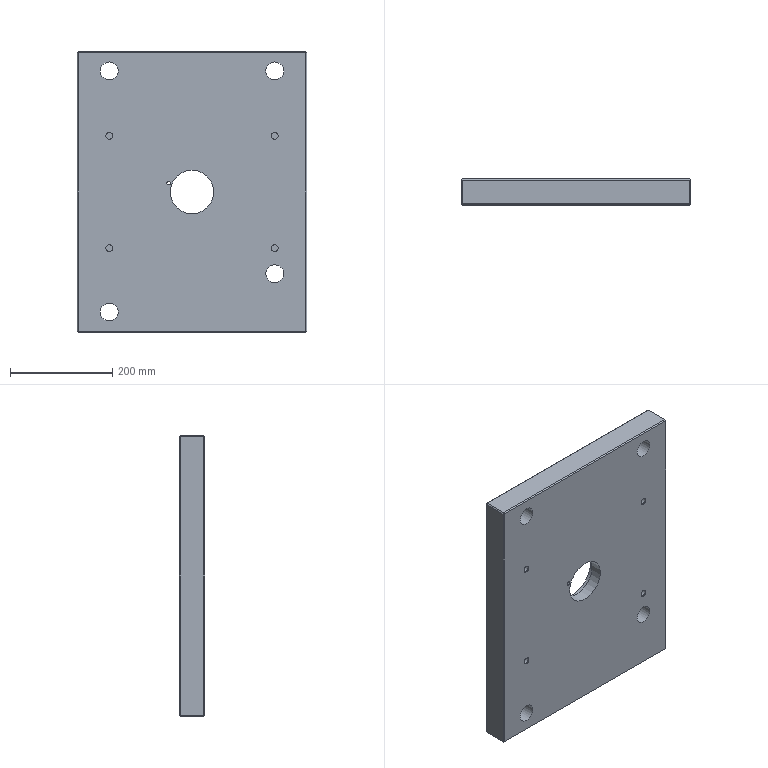Part | STEP file | TOP-CLAMP-PLATE_id506_x_t | 1 solid | 58 faces | box 450 x 50 x 550 mm | volume 11584870 mm3 | plane 29 | cylinder 21 | cone 8 | commonest cylinder face diameters 13.2 x4 16 x4 35 x4 40 x4 7 x1 12 x1
STEP:
#1=CARTESIAN_POINT('',(0.,160.5,84.487));
#2=VERTEX_POINT('',#1);
#3=CARTESIAN_POINT('',(0.,160.5,0.));
#4=DIRECTION('',(0.,1.,0.));
#5=DIRECTION('',(0.,0.,1.));
#6=AXIS2_PLACEMENT_3D('',#3,#4,#5);
#7=CIRCLE('',#6,84.487);
#8=EDGE_CURVE('',#2,#2,#7,.T.);
#9=ORIENTED_EDGE('',*,*,#8,.F.);
#10=EDGE_LOOP('',(#9));
#11=FACE_BOUND('',#10,.T.);
#12=CARTESIAN_POINT('',(0.,175.5,84.487));
#13=VERTEX_POINT('',#12);
#14=CARTESIAN_POINT('',(0.,175.5,0.));
#15=DIRECTION('',(0.,-1.,0.));
#16=DIRECTION('',(0.,0.,1.));
#17=AXIS2_PLACEMENT_3D('',#14,#15,#16);
#18=CIRCLE('',#17,84.487);
#19=EDGE_CURVE('',#13,#13,#18,.T.);
#20=ORIENTED_EDGE('',*,*,#19,.F.);
#21=EDGE_LOOP('',(#20));
#22=FACE_BOUND('',#21,.T.);
#23=CARTESIAN_POINT('',(0.,123.,0.));
#24=DIRECTION('',(0.,1.,0.));
#25=DIRECTION('',(0.,0.,1.));
#26=AXIS2_PLACEMENT_3D('',#23,#24,#25);
#27=CYLINDRICAL_SURFACE('',#26,84.487);
#28=ADVANCED_FACE('',(#11,#22),#27,.F.);
#29=CARTESIAN_POINT('',(-162.,147.5,103.));
#30=VERTEX_POINT('',#29);
#31=CARTESIAN_POINT('',(-162.,147.5,110.));
#32=DIRECTION('',(0.,-1.,0.));
#33=DIRECTION('',(0.,0.,-1.));
#34=AXIS2_PLACEMENT_3D('',#31,#32,#33);
#35=CIRCLE('',#34,7.);
#36=EDGE_CURVE('',#30,#30,#35,.T.);
#37=ORIENTED_EDGE('',*,*,#36,.T.);
#38=EDGE_LOOP('',(#37));
#39=FACE_OUTER_BOUND('',#38,.T.);
#40=CARTESIAN_POINT('',(-162.,147.5,110.));
#41=DIRECTION('',(0.,-1.,0.));
#42=DIRECTION('',(0.,0.,-1.));
#43=AXIS2_PLACEMENT_3D('',#40,#41,#42);
#44=PLANE('',#43);
#45=ADVANCED_FACE('',(#39),#44,.T.);
#46=CARTESIAN_POINT('',(-162.,147.5,-117.));
#47=VERTEX_POINT('',#46);
#48=CARTESIAN_POINT('',(-162.,147.5,-110.));
#49=DIRECTION('',(0.,-1.,0.));
#50=DIRECTION('',(0.,0.,-1.));
#51=AXIS2_PLACEMENT_3D('',#48,#49,#50);
#52=CIRCLE('',#51,7.);
#53=EDGE_CURVE('',#47,#47,#52,.T.);
#54=ORIENTED_EDGE('',*,*,#53,.T.);
#55=EDGE_LOOP('',(#54));
#56=FACE_OUTER_BOUND('',#55,.T.);
#57=CARTESIAN_POINT('',(-162.,147.5,-110.));
#58=DIRECTION('',(0.,1.,0.));
#59=DIRECTION('',(0.,0.,1.));
#60=AXIS2_PLACEMENT_3D('',#57,#58,#59);
#61=PLANE('',#60);
#62=ADVANCED_FACE('',(#56),#61,.F.);
#63=CARTESIAN_POINT('',(162.,147.5,103.));
#64=VERTEX_POINT('',#63);
#65=CARTESIAN_POINT('',(162.,147.5,110.));
#66=DIRECTION('',(0.,-1.,0.));
#67=DIRECTION('',(0.,0.,-1.));
#68=AXIS2_PLACEMENT_3D('',#65,#66,#67);
#69=CIRCLE('',#68,7.);
#70=EDGE_CURVE('',#64,#64,#69,.T.);
#71=ORIENTED_EDGE('',*,*,#70,.T.);
#72=EDGE_LOOP('',(#71));
#73=FACE_OUTER_BOUND('',#72,.T.);
#74=CARTESIAN_POINT('',(162.,147.5,110.));
#75=DIRECTION('',(0.,1.,0.));
#76=DIRECTION('',(0.,0.,1.));
#77=AXIS2_PLACEMENT_3D('',#74,#75,#76);
#78=PLANE('',#77);
#79=ADVANCED_FACE('',(#73),#78,.F.);
#80=CARTESIAN_POINT('',(162.,147.5,-117.));
#81=VERTEX_POINT('',#80);
#82=CARTESIAN_POINT('',(162.,147.5,-110.));
#83=DIRECTION('',(0.,-1.,0.));
#84=DIRECTION('',(0.,0.,-1.));
#85=AXIS2_PLACEMENT_3D('',#82,#83,#84);
#86=CIRCLE('',#85,7.);
#87=EDGE_CURVE('',#81,#81,#86,.T.);
#88=ORIENTED_EDGE('',*,*,#87,.T.);
#89=EDGE_LOOP('',(#88));
#90=FACE_OUTER_BOUND('',#89,.T.);
#91=CARTESIAN_POINT('',(162.,147.5,-110.));
#92=DIRECTION('',(0.,-1.,0.));
#93=DIRECTION('',(0.,0.,-1.));
#94=AXIS2_PLACEMENT_3D('',#91,#92,#93);
#95=PLANE('',#94);
#96=ADVANCED_FACE('',(#90),#95,.T.);
#97=ORIENTED_EDGE('',*,*,#19,.T.);
#98=EDGE_LOOP('',(#97));
#99=FACE_BOUND('',#98,.T.);
#100=CARTESIAN_POINT('',(162.,175.5,257.));
#101=VERTEX_POINT('',#100);
#102=CARTESIAN_POINT('',(162.,175.5,237.));
#103=DIRECTION('',(0.,-1.,0.));
#104=DIRECTION('',(0.,0.,1.));
#105=AXIS2_PLACEMENT_3D('',#102,#103,#104);
#106=CIRCLE('',#105,20.);
#107=EDGE_CURVE('',#101,#101,#106,.T.);
#108=ORIENTED_EDGE('',*,*,#107,.T.);
#109=EDGE_LOOP('',(#108));
#110=FACE_BOUND('',#109,.T.);
#111=CARTESIAN_POINT('',(-162.,175.5,257.));
#112=VERTEX_POINT('',#111);
#113=CARTESIAN_POINT('',(-162.,175.5,237.));
#114=DIRECTION('',(0.,-1.,0.));
#115=DIRECTION('',(0.,0.,1.));
#116=AXIS2_PLACEMENT_3D('',#113,#114,#115);
#117=CIRCLE('',#116,20.);
#118=EDGE_CURVE('',#112,#112,#117,.T.);
#119=ORIENTED_EDGE('',*,*,#118,.T.);
#120=EDGE_LOOP('',(#119));
#121=FACE_BOUND('',#120,.T.);
#122=CARTESIAN_POINT('',(-162.,175.5,-215.));
#123=VERTEX_POINT('',#122);
#124=CARTESIAN_POINT('',(-162.,175.5,-235.));
#125=DIRECTION('',(0.,-1.,0.));
#126=DIRECTION('',(0.,0.,1.));
#127=AXIS2_PLACEMENT_3D('',#124,#125,#126);
#128=CIRCLE('',#127,20.);
#129=EDGE_CURVE('',#123,#123,#128,.T.);
#130=ORIENTED_EDGE('',*,*,#129,.T.);
#131=EDGE_LOOP('',(#130));
#132=FACE_BOUND('',#131,.T.);
#133=CARTESIAN_POINT('',(162.,175.5,-140.));
#134=VERTEX_POINT('',#133);
#135=CARTESIAN_POINT('',(162.,175.5,-160.));
#136=DIRECTION('',(0.,-1.,0.));
#137=DIRECTION('',(0.,0.,1.));
#138=AXIS2_PLACEMENT_3D('',#135,#136,#137);
#139=CIRCLE('',#138,20.);
#140=EDGE_CURVE('',#134,#134,#139,.T.);
#141=ORIENTED_EDGE('',*,*,#140,.T.);
#142=EDGE_LOOP('',(#141));
#143=FACE_BOUND('',#142,.T.);
#144=CARTESIAN_POINT('',(-223.,175.5,273.));
#145=VERTEX_POINT('',#144);
#146=CARTESIAN_POINT('',(-223.,175.5,-273.));
#147=VERTEX_POINT('',#146);
#148=CARTESIAN_POINT('',(-223.,175.5,273.));
#149=DIRECTION('',(0.,0.,-1.));
#150=VECTOR('',#149,1.);
#151=LINE('',#148,#150);
#152=EDGE_CURVE('',#145,#147,#151,.T.);
#153=ORIENTED_EDGE('',*,*,#152,.F.);
#154=CARTESIAN_POINT('',(223.,175.5,273.));
#155=VERTEX_POINT('',#154);
#156=CARTESIAN_POINT('',(-225.,175.5,273.));
#157=DIRECTION('',(-1.,0.,0.));
#158=VECTOR('',#157,1.);
#159=LINE('',#156,#158);
#160=EDGE_CURVE('',#155,#145,#159,.T.);
#161=ORIENTED_EDGE('',*,*,#160,.F.);
#162=CARTESIAN_POINT('',(223.,175.5,-273.));
#163=VERTEX_POINT('',#162);
#164=CARTESIAN_POINT('',(223.,175.5,273.));
#165=DIRECTION('',(0.,0.,1.));
#166=VECTOR('',#165,1.);
#167=LINE('',#164,#166);
#168=EDGE_CURVE('',#163,#155,#167,.T.);
#169=ORIENTED_EDGE('',*,*,#168,.F.);
#170=CARTESIAN_POINT('',(-225.,175.5,-273.));
#171=DIRECTION('',(-1.,0.,0.));
#172=VECTOR('',#171,1.);
#173=LINE('',#170,#172);
#174=EDGE_CURVE('',#163,#147,#173,.T.);
#175=ORIENTED_EDGE('',*,*,#174,.T.);
#176=EDGE_LOOP('',(#153,#161,#169,#175));
#177=FACE_BOUND('',#176,.T.);
#178=CARTESIAN_POINT('',(-225.,175.5,275.));
#179=DIRECTION('',(0.,1.,0.));
#180=DIRECTION('',(0.,0.,1.));
#181=AXIS2_PLACEMENT_3D('',#178,#179,#180);
#182=PLANE('',#181);
#183=ADVANCED_FACE('',(#99,#110,#121,#132,#143,#177),#182,.T.);
#184=CARTESIAN_POINT('',(-48.524,160.5,12.058));
#185=VERTEX_POINT('',#184);
#186=CARTESIAN_POINT('',(-44.286,160.5,23.21));
#187=VERTEX_POINT('',#186);
#188=CARTESIAN_POINT('',(0.,160.5,0.));
#189=DIRECTION('',(0.,-1.,0.));
#190=DIRECTION('',(0.,0.,1.));
#191=AXIS2_PLACEMENT_3D('',#188,#189,#190);
#192=CIRCLE('',#191,50.);
#193=EDGE_CURVE('',#185,#187,#192,.T.);
#194=ORIENTED_EDGE('',*,*,#193,.T.);
#195=CARTESIAN_POINT('',(-45.804,160.5,17.406));
#196=DIRECTION('',(0.,-1.,0.));
#197=DIRECTION('',(0.,0.,1.));
#198=AXIS2_PLACEMENT_3D('',#195,#196,#197);
#199=CIRCLE('',#198,6.);
#200=EDGE_CURVE('',#187,#185,#199,.T.);
#201=ORIENTED_EDGE('',*,*,#200,.T.);
#202=EDGE_LOOP('',(#194,#201));
#203=FACE_BOUND('',#202,.T.);
#204=ORIENTED_EDGE('',*,*,#8,.T.);
#205=EDGE_LOOP('',(#204));
#206=FACE_BOUND('',#205,.T.);
#207=CARTESIAN_POINT('',(0.,160.5,0.));
#208=DIRECTION('',(0.,1.,0.));
#209=DIRECTION('',(0.,0.,1.));
#210=AXIS2_PLACEMENT_3D('',#207,#208,#209);
#211=PLANE('',#210);
#212=ADVANCED_FACE('',(#203,#206),#211,.T.);
#213=ORIENTED_EDGE('',*,*,#36,.F.);
#214=EDGE_LOOP('',(#213));
#215=FACE_BOUND('',#214,.T.);
#216=CARTESIAN_POINT('',(-162.,147.,102.));
#217=VERTEX_POINT('',#216);
#218=CARTESIAN_POINT('',(-162.,147.,110.));
#219=DIRECTION('',(0.,-1.,0.));
#220=DIRECTION('',(0.,0.,-1.));
#221=AXIS2_PLACEMENT_3D('',#218,#219,#220);
#222=CIRCLE('',#221,8.);
#223=EDGE_CURVE('',#217,#217,#222,.T.);
#224=ORIENTED_EDGE('',*,*,#223,.T.);
#225=EDGE_LOOP('',(#224));
#226=FACE_BOUND('',#225,.T.);
#227=CARTESIAN_POINT('',(-162.,147.,110.));
#228=DIRECTION('',(0.,-1.,0.));
#229=DIRECTION('',(0.,0.,-1.));
#230=AXIS2_PLACEMENT_3D('',#227,#228,#229);
#231=CONICAL_SURFACE('',#230,8.,63.435);
#232=ADVANCED_FACE('',(#215,#226),#231,.F.);
#233=ORIENTED_EDGE('',*,*,#53,.F.);
#234=EDGE_LOOP('',(#233));
#235=FACE_BOUND('',#234,.T.);
#236=CARTESIAN_POINT('',(-162.,147.,-102.));
#237=VERTEX_POINT('',#236);
#238=CARTESIAN_POINT('',(-162.,147.,-110.));
#239=DIRECTION('',(0.,-1.,0.));
#240=DIRECTION('',(0.,0.,1.));
#241=AXIS2_PLACEMENT_3D('',#238,#239,#240);
#242=CIRCLE('',#241,8.);
#243=EDGE_CURVE('',#237,#237,#242,.T.);
#244=ORIENTED_EDGE('',*,*,#243,.T.);
#245=EDGE_LOOP('',(#244));
#246=FACE_BOUND('',#245,.T.);
#247=CARTESIAN_POINT('',(-162.,147.,-110.));
#248=DIRECTION('',(0.,-1.,0.));
#249=DIRECTION('',(0.,0.,-1.));
#250=AXIS2_PLACEMENT_3D('',#247,#248,#249);
#251=CONICAL_SURFACE('',#250,8.,63.435);
#252=ADVANCED_FACE('',(#235,#246),#251,.F.);
#253=ORIENTED_EDGE('',*,*,#70,.F.);
#254=EDGE_LOOP('',(#253));
#255=FACE_BOUND('',#254,.T.);
#256=CARTESIAN_POINT('',(162.,147.,118.));
#257=VERTEX_POINT('',#256);
#258=CARTESIAN_POINT('',(162.,147.,110.));
#259=DIRECTION('',(0.,-1.,0.));
#260=DIRECTION('',(0.,0.,1.));
#261=AXIS2_PLACEMENT_3D('',#258,#259,#260);
#262=CIRCLE('',#261,8.);
#263=EDGE_CURVE('',#257,#257,#262,.T.);
#264=ORIENTED_EDGE('',*,*,#263,.T.);
#265=EDGE_LOOP('',(#264));
#266=FACE_BOUND('',#265,.T.);
#267=CARTESIAN_POINT('',(162.,147.,110.));
#268=DIRECTION('',(0.,-1.,0.));
#269=DIRECTION('',(0.,0.,-1.));
#270=AXIS2_PLACEMENT_3D('',#267,#268,#269);
#271=CONICAL_SURFACE('',#270,8.,63.435);
#272=ADVANCED_FACE('',(#255,#266),#271,.F.);
#273=CARTESIAN_POINT('',(162.,147.,-118.));
#274=VERTEX_POINT('',#273);
#275=CARTESIAN_POINT('',(162.,147.,-110.));
#276=DIRECTION('',(0.,-1.,0.));
#277=DIRECTION('',(0.,0.,-1.));
#278=AXIS2_PLACEMENT_3D('',#275,#276,#277);
#279=CIRCLE('',#278,8.);
#280=EDGE_CURVE('',#274,#274,#279,.T.);
#281=ORIENTED_EDGE('',*,*,#280,.T.);
#282=EDGE_LOOP('',(#281));
#283=FACE_BOUND('',#282,.T.);
#284=ORIENTED_EDGE('',*,*,#87,.F.);
#285=EDGE_LOOP('',(#284));
#286=FACE_BOUND('',#285,.T.);
#287=CARTESIAN_POINT('',(162.,147.,-110.));
#288=DIRECTION('',(0.,-1.,0.));
#289=DIRECTION('',(0.,0.,-1.));
#290=AXIS2_PLACEMENT_3D('',#287,#288,#289);
#291=CONICAL_SURFACE('',#290,8.,63.435);
#292=ADVANCED_FACE('',(#283,#286),#291,.F.);
#293=CARTESIAN_POINT('',(-224.,174.5,274.));
#294=VERTEX_POINT('',#293);
#295=CARTESIAN_POINT('',(-223.,175.5,273.));
#296=DIRECTION('',(-0.5774,-0.5774,0.5774));
#297=VECTOR('',#296,1.);
#298=LINE('',#295,#297);
#299=EDGE_CURVE('',#145,#294,#298,.T.);
#300=ORIENTED_EDGE('',*,*,#299,.F.);
#301=ORIENTED_EDGE('',*,*,#152,.T.);
#302=CARTESIAN_POINT('',(-224.,174.5,-274.));
#303=VERTEX_POINT('',#302);
#304=CARTESIAN_POINT('',(-223.,175.5,-273.));
#305=DIRECTION('',(-0.5774,-0.5774,-0.5774));
#306=VECTOR('',#305,1.);
#307=LINE('',#304,#306);
#308=EDGE_CURVE('',#147,#303,#307,.T.);
#309=ORIENTED_EDGE('',*,*,#308,.T.);
#310=CARTESIAN_POINT('',(-225.,173.5,-273.));
#311=VERTEX_POINT('',#310);
#312=CARTESIAN_POINT('',(-224.,174.5,-274.));
#313=DIRECTION('',(-0.5774,-0.5774,0.5774));
#314=VECTOR('',#313,1.);
#315=LINE('',#312,#314);
#316=EDGE_CURVE('',#303,#311,#315,.T.);
#317=ORIENTED_EDGE('',*,*,#316,.T.);
#318=CARTESIAN_POINT('',(-225.,173.5,273.));
#319=VERTEX_POINT('',#318);
#320=CARTESIAN_POINT('',(-225.,173.5,275.));
#321=DIRECTION('',(0.,0.,-1.));
#322=VECTOR('',#321,1.);
#323=LINE('',#320,#322);
#324=EDGE_CURVE('',#319,#311,#323,.T.);
#325=ORIENTED_EDGE('',*,*,#324,.F.);
#326=CARTESIAN_POINT('',(-224.,174.5,274.));
#327=DIRECTION('',(-0.5774,-0.5774,-0.5774));
#328=VECTOR('',#327,1.);
#329=LINE('',#326,#328);
#330=EDGE_CURVE('',#294,#319,#329,.T.);
#331=ORIENTED_EDGE('',*,*,#330,.F.);
#332=EDGE_LOOP('',(#300,#301,#309,#317,#325,#331));
#333=FACE_OUTER_BOUND('',#332,.T.);
#334=CARTESIAN_POINT('',(-223.,175.5,273.));
#335=DIRECTION('',(-0.7071,0.7071,0.));
#336=DIRECTION('',(-0.7071,-0.7071,0.));
#337=AXIS2_PLACEMENT_3D('',#334,#335,#336);
#338=PLANE('',#337);
#339=ADVANCED_FACE('',(#333),#338,.T.);
#340=CARTESIAN_POINT('',(-225.,127.5,-273.));
#341=VERTEX_POINT('',#340);
#342=CARTESIAN_POINT('',(-224.,126.5,-274.));
#343=VERTEX_POINT('',#342);
#344=CARTESIAN_POINT('',(-225.,127.5,-273.));
#345=DIRECTION('',(0.5774,-0.5774,-0.5774));
#346=VECTOR('',#345,1.);
#347=LINE('',#344,#346);
#348=EDGE_CURVE('',#341,#343,#347,.T.);
#349=ORIENTED_EDGE('',*,*,#348,.F.);
#350=CARTESIAN_POINT('',(-225.,125.5,-273.));
#351=DIRECTION('',(0.,-1.,0.));
#352=VECTOR('',#351,1.);
#353=LINE('',#350,#352);
#354=EDGE_CURVE('',#311,#341,#353,.T.);
#355=ORIENTED_EDGE('',*,*,#354,.F.);
#356=ORIENTED_EDGE('',*,*,#316,.F.);
#357=CARTESIAN_POINT('',(-223.,173.5,-275.));
#358=VERTEX_POINT('',#357);
#359=CARTESIAN_POINT('',(-224.,174.5,-274.));
#360=DIRECTION('',(0.5774,-0.5774,-0.5774));
#361=VECTOR('',#360,1.);
#362=LINE('',#359,#361);
#363=EDGE_CURVE('',#303,#358,#362,.T.);
#364=ORIENTED_EDGE('',*,*,#363,.T.);
#365=CARTESIAN_POINT('',(-223.,127.5,-275.));
#366=VERTEX_POINT('',#365);
#367=CARTESIAN_POINT('',(-223.,60.,-275.));
#368=DIRECTION('',(0.,1.,0.));
#369=VECTOR('',#368,1.);
#370=LINE('',#367,#369);
#371=EDGE_CURVE('',#366,#358,#370,.T.);
#372=ORIENTED_EDGE('',*,*,#371,.F.);
#373=CARTESIAN_POINT('',(-224.,126.5,-274.));
#374=DIRECTION('',(0.5774,0.5774,-0.5774));
#375=VECTOR('',#374,1.);
#376=LINE('',#373,#375);
#377=EDGE_CURVE('',#343,#366,#376,.T.);
#378=ORIENTED_EDGE('',*,*,#377,.F.);
#379=EDGE_LOOP('',(#349,#355,#356,#364,#372,#378));
#380=FACE_OUTER_BOUND('',#379,.T.);
#381=CARTESIAN_POINT('',(-223.,127.5,-275.));
#382=DIRECTION('',(0.7071,0.,0.7071));
#383=DIRECTION('',(0.7071,0.,-0.7071));
#384=AXIS2_PLACEMENT_3D('',#381,#382,#383);
#385=PLANE('',#384);
#386=ADVANCED_FACE('',(#380),#385,.F.);
#387=ORIENTED_EDGE('',*,*,#308,.F.);
#388=ORIENTED_EDGE('',*,*,#174,.F.);
#389=CARTESIAN_POINT('',(224.,174.5,-274.));
#390=VERTEX_POINT('',#389);
#391=CARTESIAN_POINT('',(224.,174.5,-274.));
#392=DIRECTION('',(-0.5774,0.5774,0.5774));
#393=VECTOR('',#392,1.);
#394=LINE('',#391,#393);
#395=EDGE_CURVE('',#390,#163,#394,.T.);
#396=ORIENTED_EDGE('',*,*,#395,.F.);
#397=CARTESIAN_POINT('',(223.,173.5,-275.));
#398=VERTEX_POINT('',#397);
#399=CARTESIAN_POINT('',(224.,174.5,-274.));
#400=DIRECTION('',(-0.5774,-0.5774,-0.5774));
#401=VECTOR('',#400,1.);
#402=LINE('',#399,#401);
#403=EDGE_CURVE('',#390,#398,#402,.T.);
#404=ORIENTED_EDGE('',*,*,#403,.T.);
#405=CARTESIAN_POINT('',(200.,173.5,-275.));
#406=DIRECTION('',(1.,0.,0.));
#407=VECTOR('',#406,1.);
#408=LINE('',#405,#407);
#409=EDGE_CURVE('',#358,#398,#408,.T.);
#410=ORIENTED_EDGE('',*,*,#409,.F.);
#411=ORIENTED_EDGE('',*,*,#363,.F.);
#412=EDGE_LOOP('',(#387,#388,#396,#404,#410,#411));
#413=FACE_OUTER_BOUND('',#412,.T.);
#414=CARTESIAN_POINT('',(-225.,173.5,-275.));
#415=DIRECTION('',(0.,-0.7071,0.7071));
#416=DIRECTION('',(0.,-0.7071,-0.7071));
#417=AXIS2_PLACEMENT_3D('',#414,#415,#416);
#418=PLANE('',#417);
#419=ADVANCED_FACE('',(#413),#418,.F.);
#420=CARTESIAN_POINT('',(225.,173.5,-273.));
#421=VERTEX_POINT('',#420);
#422=CARTESIAN_POINT('',(225.,173.5,-273.));
#423=DIRECTION('',(-0.5774,0.5774,-0.5774));
#424=VECTOR('',#423,1.);
#425=LINE('',#422,#424);
#426=EDGE_CURVE('',#421,#390,#425,.T.);
#427=ORIENTED_EDGE('',*,*,#426,.F.);
#428=CARTESIAN_POINT('',(225.,127.5,-273.));
#429=VERTEX_POINT('',#428);
#430=CARTESIAN_POINT('',(225.,175.5,-273.));
#431=DIRECTION('',(0.,1.,0.));
#432=VECTOR('',#431,1.);
#433=LINE('',#430,#432);
#434=EDGE_CURVE('',#429,#421,#433,.T.);
#435=ORIENTED_EDGE('',*,*,#434,.F.);
#436=CARTESIAN_POINT('',(224.,126.5,-274.));
#437=VERTEX_POINT('',#436);
#438=CARTESIAN_POINT('',(224.,126.5,-274.));
#439=DIRECTION('',(0.5774,0.5774,0.5774));
#440=VECTOR('',#439,1.);
#441=LINE('',#438,#440);
#442=EDGE_CURVE('',#437,#429,#441,.T.);
#443=ORIENTED_EDGE('',*,*,#442,.F.);
#444=CARTESIAN_POINT('',(223.,127.5,-275.));
#445=VERTEX_POINT('',#444);
#446=CARTESIAN_POINT('',(223.,127.5,-275.));
#447=DIRECTION('',(0.5774,-0.5774,0.5774));
#448=VECTOR('',#447,1.);
#449=LINE('',#446,#448);
#450=EDGE_CURVE('',#445,#437,#449,.T.);
#451=ORIENTED_EDGE('',*,*,#450,.F.);
#452=CARTESIAN_POINT('',(223.,60.,-275.));
#453=DIRECTION('',(0.,-1.,0.));
#454=VECTOR('',#453,1.);
#455=LINE('',#452,#454);
#456=EDGE_CURVE('',#398,#445,#455,.T.);
#457=ORIENTED_EDGE('',*,*,#456,.F.);
#458=ORIENTED_EDGE('',*,*,#403,.F.);
#459=EDGE_LOOP('',(#427,#435,#443,#451,#457,#458));
#460=FACE_OUTER_BOUND('',#459,.T.);
#461=CARTESIAN_POINT('',(223.,175.5,-275.));
#462=DIRECTION('',(-0.7071,0.,0.7071));
#463=DIRECTION('',(0.7071,0.,0.7071));
#464=AXIS2_PLACEMENT_3D('',#461,#462,#463);
#465=PLANE('',#464);
#466=ADVANCED_FACE('',(#460),#465,.F.);
#467=CARTESIAN_POINT('',(225.,173.5,273.));
#468=VERTEX_POINT('',#467);
#469=CARTESIAN_POINT('',(224.,174.5,274.));
#470=VERTEX_POINT('',#469);
#471=CARTESIAN_POINT('',(225.,173.5,273.));
#472=DIRECTION('',(-0.5774,0.5774,0.5774));
#473=VECTOR('',#472,1.);
#474=LINE('',#471,#473);
#475=EDGE_CURVE('',#468,#470,#474,.T.);
#476=ORIENTED_EDGE('',*,*,#475,.F.);
#477=CARTESIAN_POINT('',(225.,173.5,275.));
#478=DIRECTION('',(0.,0.,1.));
#479=VECTOR('',#478,1.);
#480=LINE('',#477,#479);
#481=EDGE_CURVE('',#421,#468,#480,.T.);
#482=ORIENTED_EDGE('',*,*,#481,.F.);
#483=ORIENTED_EDGE('',*,*,#426,.T.);
#484=ORIENTED_EDGE('',*,*,#395,.T.);
#485=ORIENTED_EDGE('',*,*,#168,.T.);
#486=CARTESIAN_POINT('',(224.,174.5,274.));
#487=DIRECTION('',(-0.5774,0.5774,-0.5774));
#488=VECTOR('',#487,1.);
#489=LINE('',#486,#488);
#490=EDGE_CURVE('',#470,#155,#489,.T.);
#491=ORIENTED_EDGE('',*,*,#490,.F.);
#492=EDGE_LOOP('',(#476,#482,#483,#484,#485,#491));
#493=FACE_OUTER_BOUND('',#492,.T.);
#494=CARTESIAN_POINT('',(225.,173.5,273.));
#495=DIRECTION('',(0.7071,0.7071,0.));
#496=DIRECTION('',(-0.7071,0.7071,0.));
#497=AXIS2_PLACEMENT_3D('',#494,#495,#496);
#498=PLANE('',#497);
#499=ADVANCED_FACE('',(#493),#498,.T.);
#500=CARTESIAN_POINT('',(-224.,126.5,274.));
#501=VERTEX_POINT('',#500);
#502=CARTESIAN_POINT('',(-223.,127.5,275.));
#503=VERTEX_POINT('',#502);
#504=CARTESIAN_POINT('',(-224.,126.5,274.));
#505=DIRECTION('',(0.5774,0.5774,0.5774));
#506=VECTOR('',#505,1.);
#507=LINE('',#504,#506);
#508=EDGE_CURVE('',#501,#503,#507,.T.);
#509=ORIENTED_EDGE('',*,*,#508,.T.);
#510=CARTESIAN_POINT('',(-223.,173.5,275.));
#511=VERTEX_POINT('',#510);
#512=CARTESIAN_POINT('',(-223.,90.5,275.));
#513=DIRECTION('',(0.,1.,0.));
#514=VECTOR('',#513,1.);
#515=LINE('',#512,#514);
#516=EDGE_CURVE('',#503,#511,#515,.T.);
#517=ORIENTED_EDGE('',*,*,#516,.T.);
#518=CARTESIAN_POINT('',(-224.,174.5,274.));
#519=DIRECTION('',(0.5774,-0.5774,0.5774));
#520=VECTOR('',#519,1.);
#521=LINE('',#518,#520);
#522=EDGE_CURVE('',#294,#511,#521,.T.);
#523=ORIENTED_EDGE('',*,*,#522,.F.);
#524=ORIENTED_EDGE('',*,*,#330,.T.);
#525=CARTESIAN_POINT('',(-225.,127.5,273.));
#526=VERTEX_POINT('',#525);
#527=CARTESIAN_POINT('',(-225.,125.5,273.));
#528=DIRECTION('',(0.,1.,0.));
#529=VECTOR('',#528,1.);
#530=LINE('',#527,#529);
#531=EDGE_CURVE('',#526,#319,#530,.T.);
#532=ORIENTED_EDGE('',*,*,#531,.F.);
#533=CARTESIAN_POINT('',(-225.,127.5,273.));
#534=DIRECTION('',(0.5774,-0.5774,0.5774));
#535=VECTOR('',#534,1.);
#536=LINE('',#533,#535);
#537=EDGE_CURVE('',#526,#501,#536,.T.);
#538=ORIENTED_EDGE('',*,*,#537,.T.);
#539=EDGE_LOOP('',(#509,#517,#523,#524,#532,#538));
#540=FACE_OUTER_BOUND('',#539,.T.);
#541=CARTESIAN_POINT('',(-223.,127.5,275.));
#542=DIRECTION('',(-0.7071,0.,0.7071));
#543=DIRECTION('',(0.7071,0.,0.7071));
#544=AXIS2_PLACEMENT_3D('',#541,#542,#543);
#545=PLANE('',#544);
#546=ADVANCED_FACE('',(#540),#545,.T.);
#547=ORIENTED_EDGE('',*,*,#522,.T.);
#548=CARTESIAN_POINT('',(223.,173.5,275.));
#549=VERTEX_POINT('',#548);
#550=CARTESIAN_POINT('',(-200.,173.5,275.));
#551=DIRECTION('',(1.,0.,0.));
#552=VECTOR('',#551,1.);
#553=LINE('',#550,#552);
#554=EDGE_CURVE('',#511,#549,#553,.T.);
#555=ORIENTED_EDGE('',*,*,#554,.T.);
#556=CARTESIAN_POINT('',(224.,174.5,274.));
#557=DIRECTION('',(-0.5774,-0.5774,0.5774));
#558=VECTOR('',#557,1.);
#559=LINE('',#556,#558);
#560=EDGE_CURVE('',#470,#549,#559,.T.);
#561=ORIENTED_EDGE('',*,*,#560,.F.);
#562=ORIENTED_EDGE('',*,*,#490,.T.);
#563=ORIENTED_EDGE('',*,*,#160,.T.);
#564=ORIENTED_EDGE('',*,*,#299,.T.);
#565=EDGE_LOOP('',(#547,#555,#561,#562,#563,#564));
#566=FACE_OUTER_BOUND('',#565,.T.);
#567=CARTESIAN_POINT('',(-225.,173.5,275.));
#568=DIRECTION('',(0.,0.7071,0.7071));
#569=DIRECTION('',(0.,-0.7071,0.7071));
#570=AXIS2_PLACEMENT_3D('',#567,#568,#569);
#571=PLANE('',#570);
#572=ADVANCED_FACE('',(#566),#571,.T.);
#573=ORIENTED_EDGE('',*,*,#560,.T.);
#574=CARTESIAN_POINT('',(223.,127.5,275.));
#575=VERTEX_POINT('',#574);
#576=CARTESIAN_POINT('',(223.,90.5,275.));
#577=DIRECTION('',(0.,-1.,0.));
#578=VECTOR('',#577,1.);
#579=LINE('',#576,#578);
#580=EDGE_CURVE('',#549,#575,#579,.T.);
#581=ORIENTED_EDGE('',*,*,#580,.T.);
#582=CARTESIAN_POINT('',(224.,126.5,274.));
#583=VERTEX_POINT('',#582);
#584=CARTESIAN_POINT('',(223.,127.5,275.));
#585=DIRECTION('',(0.5774,-0.5774,-0.5774));
#586=VECTOR('',#585,1.);
#587=LINE('',#584,#586);
#588=EDGE_CURVE('',#575,#583,#587,.T.);
#589=ORIENTED_EDGE('',*,*,#588,.T.);
#590=CARTESIAN_POINT('',(225.,127.5,273.));
#591=VERTEX_POINT('',#590);
#592=CARTESIAN_POINT('',(224.,126.5,274.));
#593=DIRECTION('',(0.5774,0.5774,-0.5774));
#594=VECTOR('',#593,1.);
#595=LINE('',#592,#594);
#596=EDGE_CURVE('',#583,#591,#595,.T.);
#597=ORIENTED_EDGE('',*,*,#596,.T.);
#598=CARTESIAN_POINT('',(225.,175.5,273.));
#599=DIRECTION('',(0.,-1.,0.));
#600=VECTOR('',#599,1.);
#601=LINE('',#598,#600);
#602=EDGE_CURVE('',#468,#591,#601,.T.);
#603=ORIENTED_EDGE('',*,*,#602,.F.);
#604=ORIENTED_EDGE('',*,*,#475,.T.);
#605=EDGE_LOOP('',(#573,#581,#589,#597,#603,#604));
#606=FACE_OUTER_BOUND('',#605,.T.);
#607=CARTESIAN_POINT('',(223.,175.5,275.));
#608=DIRECTION('',(0.7071,0.,0.7071));
#609=DIRECTION('',(0.7071,0.,-0.7071));
#610=AXIS2_PLACEMENT_3D('',#607,#608,#609);
#611=PLANE('',#610);
#612=ADVANCED_FACE('',(#606),#611,.T.);
#613=CARTESIAN_POINT('',(-162.,167.5,-215.));
#614=VERTEX_POINT('',#613);
#615=CARTESIAN_POINT('',(-162.,167.5,-235.));
#616=DIRECTION('',(0.,1.,0.));
#617=DIRECTION('',(0.,0.,1.));
#618=AXIS2_PLACEMENT_3D('',#615,#616,#617);
#619=CIRCLE('',#618,20.);
#620=EDGE_CURVE('',#614,#614,#619,.T.);
#621=ORIENTED_EDGE('',*,*,#620,.F.);
#622=EDGE_LOOP('',(#621));
#623=FACE_BOUND('',#622,.T.);
#624=ORIENTED_EDGE('',*,*,#129,.F.);
#625=EDGE_LOOP('',(#624));
#626=FACE_BOUND('',#625,.T.);
#627=CARTESIAN_POINT('',(-162.,175.5,-235.));
#628=DIRECTION('',(0.,1.,0.));
#629=DIRECTION('',(0.,0.,1.));
#630=AXIS2_PLACEMENT_3D('',#627,#628,#629);
#631=CYLINDRICAL_SURFACE('',#630,20.);
#632=ADVANCED_FACE('',(#623,#626),#631,.F.);
#633=CARTESIAN_POINT('',(162.,167.5,-140.));
#634=VERTEX_POINT('',#633);
#635=CARTESIAN_POINT('',(162.,167.5,-160.));
#636=DIRECTION('',(0.,1.,0.));
#637=DIRECTION('',(0.,0.,1.));
#638=AXIS2_PLACEMENT_3D('',#635,#636,#637);
#639=CIRCLE('',#638,20.);
#640=EDGE_CURVE('',#634,#634,#639,.T.);
#641=ORIENTED_EDGE('',*,*,#640,.F.);
#642=EDGE_LOOP('',(#641));
#643=FACE_BOUND('',#642,.T.);
#644=ORIENTED_EDGE('',*,*,#140,.F.);
#645=EDGE_LOOP('',(#644));
#646=FACE_BOUND('',#645,.T.);
#647=CARTESIAN_POINT('',(162.,175.5,-160.));
#648=DIRECTION('',(0.,1.,0.));
#649=DIRECTION('',(0.,0.,1.));
#650=AXIS2_PLACEMENT_3D('',#647,#648,#649);
#651=CYLINDRICAL_SURFACE('',#650,20.);
#652=ADVANCED_FACE('',(#643,#646),#651,.F.);
#653=CARTESIAN_POINT('',(162.,167.5,257.));
#654=VERTEX_POINT('',#653);
#655=CARTESIAN_POINT('',(162.,167.5,237.));
#656=DIRECTION('',(0.,1.,0.));
#657=DIRECTION('',(0.,0.,1.));
#658=AXIS2_PLACEMENT_3D('',#655,#656,#657);
#659=CIRCLE('',#658,20.);
#660=EDGE_CURVE('',#654,#654,#659,.T.);
#661=ORIENTED_EDGE('',*,*,#660,.F.);
#662=EDGE_LOOP('',(#661));
#663=FACE_BOUND('',#662,.T.);
#664=ORIENTED_EDGE('',*,*,#107,.F.);
#665=EDGE_LOOP('',(#664));
#666=FACE_BOUND('',#665,.T.);
#667=CARTESIAN_POINT('',(162.,175.5,237.));
#668=DIRECTION('',(0.,1.,0.));
#669=DIRECTION('',(0.,0.,1.));
#670=AXIS2_PLACEMENT_3D('',#667,#668,#669);
#671=CYLINDRICAL_SURFACE('',#670,20.);
#672=ADVANCED_FACE('',(#663,#666),#671,.F.);
#673=CARTESIAN_POINT('',(-162.,167.5,257.));
#674=VERTEX_POINT('',#673);
#675=CARTESIAN_POINT('',(-162.,167.5,237.));
#676=DIRECTION('',(0.,1.,0.));
#677=DIRECTION('',(0.,0.,1.));
#678=AXIS2_PLACEMENT_3D('',#675,#676,#677);
#679=CIRCLE('',#678,20.);
#680=EDGE_CURVE('',#674,#674,#679,.T.);
#681=ORIENTED_EDGE('',*,*,#680,.F.);
#682=EDGE_LOOP('',(#681));
#683=FACE_BOUND('',#682,.T.);
#684=ORIENTED_EDGE('',*,*,#118,.F.);
#685=EDGE_LOOP('',(#684));
#686=FACE_BOUND('',#685,.T.);
#687=CARTESIAN_POINT('',(-162.,175.5,237.));
#688=DIRECTION('',(0.,1.,0.));
#689=DIRECTION('',(0.,0.,1.));
#690=AXIS2_PLACEMENT_3D('',#687,#688,#689);
#691=CYLINDRICAL_SURFACE('',#690,20.);
#692=ADVANCED_FACE('',(#683,#686),#691,.F.);
#693=ORIENTED_EDGE('',*,*,#193,.F.);
#694=CARTESIAN_POINT('',(-48.524,148.5,12.058));
#695=VERTEX_POINT('',#694);
#696=CARTESIAN_POINT('',(-48.524,84.975,12.058));
#697=DIRECTION('',(0.,-1.,0.));
#698=VECTOR('',#697,1.);
#699=LINE('',#696,#698);
#700=EDGE_CURVE('',#185,#695,#699,.T.);
#701=ORIENTED_EDGE('',*,*,#700,.T.);
#702=CARTESIAN_POINT('',(-44.286,148.5,23.21));
#703=VERTEX_POINT('',#702);
#704=CARTESIAN_POINT('',(0.,148.5,0.));
#705=DIRECTION('',(0.,1.,0.));
#706=DIRECTION('',(0.,0.,1.));
#707=AXIS2_PLACEMENT_3D('',#704,#705,#706);
#708=CIRCLE('',#707,50.);
#709=EDGE_CURVE('',#703,#695,#708,.T.);
#710=ORIENTED_EDGE('',*,*,#709,.F.);
#711=CARTESIAN_POINT('',(-44.286,84.975,23.21));
#712=DIRECTION('',(0.,1.,0.));
#713=VECTOR('',#712,1.);
#714=LINE('',#711,#713);
#715=EDGE_CURVE('',#703,#187,#714,.T.);
#716=ORIENTED_EDGE('',*,*,#715,.T.);
#717=EDGE_LOOP('',(#693,#701,#710,#716));
#718=FACE_OUTER_BOUND('',#717,.T.);
#719=CARTESIAN_POINT('',(0.,123.,0.));
#720=DIRECTION('',(0.,1.,0.));
#721=DIRECTION('',(0.,0.,1.));
#722=AXIS2_PLACEMENT_3D('',#719,#720,#721);
#723=CYLINDRICAL_SURFACE('',#722,50.);
#724=ADVANCED_FACE('',(#718),#723,.F.);
#725=CARTESIAN_POINT('',(-45.804,143.5,23.406));
#726=VERTEX_POINT('',#725);
#727=CARTESIAN_POINT('',(-45.804,143.5,17.406));
#728=DIRECTION('',(0.,1.,0.));
#729=DIRECTION('',(0.,0.,1.));
#730=AXIS2_PLACEMENT_3D('',#727,#728,#729);
#731=CIRCLE('',#730,6.);
#732=EDGE_CURVE('',#726,#726,#731,.T.);
#733=ORIENTED_EDGE('',*,*,#732,.F.);
#734=EDGE_LOOP('',(#733));
#735=FACE_BOUND('',#734,.T.);
#736=ORIENTED_EDGE('',*,*,#715,.F.);
#737=CARTESIAN_POINT('',(-45.804,148.5,17.406));
#738=DIRECTION('',(0.,-1.,0.));
#739=DIRECTION('',(0.,0.,1.));
#740=AXIS2_PLACEMENT_3D('',#737,#738,#739);
#741=CIRCLE('',#740,6.);
#742=EDGE_CURVE('',#695,#703,#741,.T.);
#743=ORIENTED_EDGE('',*,*,#742,.F.);
#744=ORIENTED_EDGE('',*,*,#700,.F.);
#745=ORIENTED_EDGE('',*,*,#200,.F.);
#746=EDGE_LOOP('',(#736,#743,#744,#745));
#747=FACE_BOUND('',#746,.T.);
#748=CARTESIAN_POINT('',(-45.804,84.975,17.406));
#749=DIRECTION('',(0.,1.,0.));
#750=DIRECTION('',(0.,0.,1.));
#751=AXIS2_PLACEMENT_3D('',#748,#749,#750);
#752=CYLINDRICAL_SURFACE('',#751,6.);
#753=ADVANCED_FACE('',(#735,#747),#752,.F.);
#754=ORIENTED_EDGE('',*,*,#223,.F.);
#755=EDGE_LOOP('',(#754));
#756=FACE_BOUND('',#755,.T.);
#757=CARTESIAN_POINT('',(-154.,128.45,110.));
#758=VERTEX_POINT('',#757);
#759=CARTESIAN_POINT('',(-162.,128.45,110.));
#760=DIRECTION('',(0.,-1.,0.));
#761=DIRECTION('',(1.,0.,0.));
#762=AXIS2_PLACEMENT_3D('',#759,#760,#761);
#763=CIRCLE('',#762,8.);
#764=EDGE_CURVE('',#758,#758,#763,.T.);
#765=ORIENTED_EDGE('',*,*,#764,.T.);
#766=EDGE_LOOP('',(#765));
#767=FACE_BOUND('',#766,.T.);
#768=CARTESIAN_POINT('',(-162.,72.95,110.));
#769=DIRECTION('',(0.,-1.,0.));
#770=DIRECTION('',(0.,0.,-1.));
#771=AXIS2_PLACEMENT_3D('',#768,#769,#770);
#772=CYLINDRICAL_SURFACE('',#771,8.);
#773=ADVANCED_FACE('',(#756,#767),#772,.F.);
#774=ORIENTED_EDGE('',*,*,#243,.F.);
#775=EDGE_LOOP('',(#774));
#776=FACE_BOUND('',#775,.T.);
#777=CARTESIAN_POINT('',(-170.,128.45,-110.));
#778=VERTEX_POINT('',#777);
#779=CARTESIAN_POINT('',(-162.,128.45,-110.));
#780=DIRECTION('',(0.,-1.,0.));
#781=DIRECTION('',(-1.,0.,0.));
#782=AXIS2_PLACEMENT_3D('',#779,#780,#781);
#783=CIRCLE('',#782,8.);
#784=EDGE_CURVE('',#778,#778,#783,.T.);
#785=ORIENTED_EDGE('',*,*,#784,.T.);
#786=EDGE_LOOP('',(#785));
#787=FACE_BOUND('',#786,.T.);
#788=CARTESIAN_POINT('',(-162.,72.95,-110.));
#789=DIRECTION('',(0.,1.,0.));
#790=DIRECTION('',(0.,0.,1.));
#791=AXIS2_PLACEMENT_3D('',#788,#789,#790);
#792=CYLINDRICAL_SURFACE('',#791,8.);
#793=ADVANCED_FACE('',(#776,#787),#792,.F.);
#794=ORIENTED_EDGE('',*,*,#263,.F.);
#795=EDGE_LOOP('',(#794));
#796=FACE_BOUND('',#795,.T.);
#797=CARTESIAN_POINT('',(170.,128.45,110.));
#798=VERTEX_POINT('',#797);
#799=CARTESIAN_POINT('',(162.,128.45,110.));
#800=DIRECTION('',(0.,-1.,0.));
#801=DIRECTION('',(1.,0.,0.));
#802=AXIS2_PLACEMENT_3D('',#799,#800,#801);
#803=CIRCLE('',#802,8.);
#804=EDGE_CURVE('',#798,#798,#803,.T.);
#805=ORIENTED_EDGE('',*,*,#804,.T.);
#806=EDGE_LOOP('',(#805));
#807=FACE_BOUND('',#806,.T.);
#808=CARTESIAN_POINT('',(162.,72.95,110.));
#809=DIRECTION('',(0.,1.,0.));
#810=DIRECTION('',(0.,0.,1.));
#811=AXIS2_PLACEMENT_3D('',#808,#809,#810);
#812=CYLINDRICAL_SURFACE('',#811,8.);
#813=ADVANCED_FACE('',(#796,#807),#812,.F.);
#814=CARTESIAN_POINT('',(154.,128.45,-110.));
#815=VERTEX_POINT('',#814);
#816=CARTESIAN_POINT('',(162.,128.45,-110.));
#817=DIRECTION('',(0.,-1.,0.));
#818=DIRECTION('',(-1.,0.,0.));
#819=AXIS2_PLACEMENT_3D('',#816,#817,#818);
#820=CIRCLE('',#819,8.);
#821=EDGE_CURVE('',#815,#815,#820,.T.);
#822=ORIENTED_EDGE('',*,*,#821,.T.);
#823=EDGE_LOOP('',(#822));
#824=FACE_BOUND('',#823,.T.);
#825=ORIENTED_EDGE('',*,*,#280,.F.);
#826=EDGE_LOOP('',(#825));
#827=FACE_BOUND('',#826,.T.);
#828=CARTESIAN_POINT('',(162.,72.95,-110.));
#829=DIRECTION('',(0.,-1.,0.));
#830=DIRECTION('',(0.,0.,-1.));
#831=AXIS2_PLACEMENT_3D('',#828,#829,#830);
#832=CYLINDRICAL_SURFACE('',#831,8.);
#833=ADVANCED_FACE('',(#824,#827),#832,.F.);
#834=CARTESIAN_POINT('',(-225.,127.5,273.));
#835=DIRECTION('',(0.,0.,-1.));
#836=VECTOR('',#835,1.);
#837=LINE('',#834,#836);
#838=EDGE_CURVE('',#526,#341,#837,.T.);
#839=ORIENTED_EDGE('',*,*,#838,.F.);
#840=ORIENTED_EDGE('',*,*,#531,.T.);
#841=ORIENTED_EDGE('',*,*,#324,.T.);
#842=ORIENTED_EDGE('',*,*,#354,.T.);
#843=EDGE_LOOP('',(#839,#840,#841,#842));
#844=FACE_OUTER_BOUND('',#843,.T.);
#845=CARTESIAN_POINT('',(-225.,125.5,275.));
#846=DIRECTION('',(-1.,0.,0.));
#847=DIRECTION('',(0.,0.,1.));
#848=AXIS2_PLACEMENT_3D('',#845,#846,#847);
#849=PLANE('',#848);
#850=ADVANCED_FACE('',(#844),#849,.T.);
#851=ORIENTED_EDGE('',*,*,#456,.T.);
#852=CARTESIAN_POINT('',(223.,127.5,-275.));
#853=DIRECTION('',(-1.,0.,0.));
#854=VECTOR('',#853,1.);
#855=LINE('',#852,#854);
#856=EDGE_CURVE('',#445,#366,#855,.T.);
#857=ORIENTED_EDGE('',*,*,#856,.T.);
#858=ORIENTED_EDGE('',*,*,#371,.T.);
#859=ORIENTED_EDGE('',*,*,#409,.T.);
#860=EDGE_LOOP('',(#851,#857,#858,#859));
#861=FACE_OUTER_BOUND('',#860,.T.);
#862=CARTESIAN_POINT('',(200.,60.,-275.));
#863=DIRECTION('',(0.,0.,-1.));
#864=DIRECTION('',(-1.,0.,0.));
#865=AXIS2_PLACEMENT_3D('',#862,#863,#864);
#866=PLANE('',#865);
#867=ADVANCED_FACE('',(#861),#866,.T.);
#868=ORIENTED_EDGE('',*,*,#481,.T.);
#869=ORIENTED_EDGE('',*,*,#602,.T.);
#870=CARTESIAN_POINT('',(225.,127.5,273.));
#871=DIRECTION('',(0.,0.,1.));
#872=VECTOR('',#871,1.);
#873=LINE('',#870,#872);
#874=EDGE_CURVE('',#429,#591,#873,.T.);
#875=ORIENTED_EDGE('',*,*,#874,.F.);
#876=ORIENTED_EDGE('',*,*,#434,.T.);
#877=EDGE_LOOP('',(#868,#869,#875,#876));
#878=FACE_OUTER_BOUND('',#877,.T.);
#879=CARTESIAN_POINT('',(225.,175.5,275.));
#880=DIRECTION('',(1.,0.,0.));
#881=DIRECTION('',(0.,0.,-1.));
#882=AXIS2_PLACEMENT_3D('',#879,#880,#881);
#883=PLANE('',#882);
#884=ADVANCED_FACE('',(#878),#883,.T.);
#885=ORIENTED_EDGE('',*,*,#554,.F.);
#886=ORIENTED_EDGE('',*,*,#516,.F.);
#887=CARTESIAN_POINT('',(223.,127.5,275.));
#888=DIRECTION('',(-1.,0.,0.));
#889=VECTOR('',#888,1.);
#890=LINE('',#887,#889);
#891=EDGE_CURVE('',#575,#503,#890,.T.);
#892=ORIENTED_EDGE('',*,*,#891,.F.);
#893=ORIENTED_EDGE('',*,*,#580,.F.);
#894=EDGE_LOOP('',(#885,#886,#892,#893));
#895=FACE_OUTER_BOUND('',#894,.T.);
#896=CARTESIAN_POINT('',(-200.,90.5,275.));
#897=DIRECTION('',(0.,0.,-1.));
#898=DIRECTION('',(-1.,0.,0.));
#899=AXIS2_PLACEMENT_3D('',#896,#897,#898);
#900=PLANE('',#899);
#901=ADVANCED_FACE('',(#895),#900,.F.);
#902=CARTESIAN_POINT('',(-162.,167.5,-252.5));
#903=VERTEX_POINT('',#902);
#904=CARTESIAN_POINT('',(-162.,167.5,-235.));
#905=DIRECTION('',(0.,-1.,0.));
#906=DIRECTION('',(0.,0.,-1.));
#907=AXIS2_PLACEMENT_3D('',#904,#905,#906);
#908=CIRCLE('',#907,17.5);
#909=EDGE_CURVE('',#903,#903,#908,.T.);
#910=ORIENTED_EDGE('',*,*,#909,.T.);
#911=EDGE_LOOP('',(#910));
#912=FACE_BOUND('',#911,.T.);
#913=ORIENTED_EDGE('',*,*,#620,.T.);
#914=EDGE_LOOP('',(#913));
#915=FACE_BOUND('',#914,.T.);
#916=CARTESIAN_POINT('',(-200.,167.5,275.));
#917=DIRECTION('',(0.,1.,0.));
#918=DIRECTION('',(0.,0.,1.));
#919=AXIS2_PLACEMENT_3D('',#916,#917,#918);
#920=PLANE('',#919);
#921=ADVANCED_FACE('',(#912,#915),#920,.T.);
#922=CARTESIAN_POINT('',(162.,167.5,-177.5));
#923=VERTEX_POINT('',#922);
#924=CARTESIAN_POINT('',(162.,167.5,-160.));
#925=DIRECTION('',(0.,-1.,0.));
#926=DIRECTION('',(0.,0.,-1.));
#927=AXIS2_PLACEMENT_3D('',#924,#925,#926);
#928=CIRCLE('',#927,17.5);
#929=EDGE_CURVE('',#923,#923,#928,.T.);
#930=ORIENTED_EDGE('',*,*,#929,.T.);
#931=EDGE_LOOP('',(#930));
#932=FACE_BOUND('',#931,.T.);
#933=ORIENTED_EDGE('',*,*,#640,.T.);
#934=EDGE_LOOP('',(#933));
#935=FACE_BOUND('',#934,.T.);
#936=CARTESIAN_POINT('',(-200.,167.5,275.));
#937=DIRECTION('',(0.,1.,0.));
#938=DIRECTION('',(0.,0.,1.));
#939=AXIS2_PLACEMENT_3D('',#936,#937,#938);
#940=PLANE('',#939);
#941=ADVANCED_FACE('',(#932,#935),#940,.T.);
#942=CARTESIAN_POINT('',(162.,167.5,219.5));
#943=VERTEX_POINT('',#942);
#944=CARTESIAN_POINT('',(162.,167.5,237.));
#945=DIRECTION('',(0.,-1.,0.));
#946=DIRECTION('',(0.,0.,-1.));
#947=AXIS2_PLACEMENT_3D('',#944,#945,#946);
#948=CIRCLE('',#947,17.5);
#949=EDGE_CURVE('',#943,#943,#948,.T.);
#950=ORIENTED_EDGE('',*,*,#949,.T.);
#951=EDGE_LOOP('',(#950));
#952=FACE_BOUND('',#951,.T.);
#953=ORIENTED_EDGE('',*,*,#660,.T.);
#954=EDGE_LOOP('',(#953));
#955=FACE_BOUND('',#954,.T.);
#956=CARTESIAN_POINT('',(-200.,167.5,275.));
#957=DIRECTION('',(0.,1.,0.));
#958=DIRECTION('',(0.,0.,1.));
#959=AXIS2_PLACEMENT_3D('',#956,#957,#958);
#960=PLANE('',#959);
#961=ADVANCED_FACE('',(#952,#955),#960,.T.);
#962=CARTESIAN_POINT('',(-162.,167.5,219.5));
#963=VERTEX_POINT('',#962);
#964=CARTESIAN_POINT('',(-162.,167.5,237.));
#965=DIRECTION('',(0.,-1.,0.));
#966=DIRECTION('',(0.,0.,-1.));
#967=AXIS2_PLACEMENT_3D('',#964,#965,#966);
#968=CIRCLE('',#967,17.5);
#969=EDGE_CURVE('',#963,#963,#968,.T.);
#970=ORIENTED_EDGE('',*,*,#969,.T.);
#971=EDGE_LOOP('',(#970));
#972=FACE_BOUND('',#971,.T.);
#973=ORIENTED_EDGE('',*,*,#680,.T.);
#974=EDGE_LOOP('',(#973));
#975=FACE_BOUND('',#974,.T.);
#976=CARTESIAN_POINT('',(-200.,167.5,275.));
#977=DIRECTION('',(0.,1.,0.));
#978=DIRECTION('',(0.,0.,1.));
#979=AXIS2_PLACEMENT_3D('',#976,#977,#978);
#980=PLANE('',#979);
#981=ADVANCED_FACE('',(#972,#975),#980,.T.);
#982=CARTESIAN_POINT('',(0.,148.5,42.5));
#983=VERTEX_POINT('',#982);
#984=CARTESIAN_POINT('',(0.,148.5,0.));
#985=DIRECTION('',(0.,-1.,0.));
#986=DIRECTION('',(0.,0.,1.));
#987=AXIS2_PLACEMENT_3D('',#984,#985,#986);
#988=CIRCLE('',#987,42.5);
#989=EDGE_CURVE('',#983,#983,#988,.T.);
#990=ORIENTED_EDGE('',*,*,#989,.T.);
#991=EDGE_LOOP('',(#990));
#992=FACE_BOUND('',#991,.T.);
#993=ORIENTED_EDGE('',*,*,#709,.T.);
#994=ORIENTED_EDGE('',*,*,#742,.T.);
#995=EDGE_LOOP('',(#993,#994));
#996=FACE_BOUND('',#995,.T.);
#997=CARTESIAN_POINT('',(0.,148.5,0.));
#998=DIRECTION('',(0.,1.,0.));
#999=DIRECTION('',(0.,0.,1.));
#1000=AXIS2_PLACEMENT_3D('',#997,#998,#999);
#1001=PLANE('',#1000);
#1002=ADVANCED_FACE('',(#992,#996),#1001,.T.);
#1003=CARTESIAN_POINT('',(-45.804,143.5,20.906));
#1004=VERTEX_POINT('',#1003);
#1005=CARTESIAN_POINT('',(-45.804,143.5,17.406));
#1006=DIRECTION('',(0.,-1.,0.));
#1007=DIRECTION('',(0.,0.,1.));
#1008=AXIS2_PLACEMENT_3D('',#1005,#1006,#1007);
#1009=CIRCLE('',#1008,3.5);
#1010=EDGE_CURVE('',#1004,#1004,#1009,.T.);
#1011=ORIENTED_EDGE('',*,*,#1010,.T.);
#1012=EDGE_LOOP('',(#1011));
#1013=FACE_BOUND('',#1012,.T.);
#1014=ORIENTED_EDGE('',*,*,#732,.T.);
#1015=EDGE_LOOP('',(#1014));
#1016=FACE_BOUND('',#1015,.T.);
#1017=CARTESIAN_POINT('',(-45.804,143.5,17.406));
#1018=DIRECTION('',(0.,1.,0.));
#1019=DIRECTION('',(0.,0.,1.));
#1020=AXIS2_PLACEMENT_3D('',#1017,#1018,#1019);
#1021=PLANE('',#1020);
#1022=ADVANCED_FACE('',(#1013,#1016),#1021,.T.);
#1023=ORIENTED_EDGE('',*,*,#764,.F.);
#1024=EDGE_LOOP('',(#1023));
#1025=FACE_BOUND('',#1024,.T.);
#1026=CARTESIAN_POINT('',(-162.,127.642,103.4));
#1027=VERTEX_POINT('',#1026);
#1028=CARTESIAN_POINT('',(-162.,127.642,110.));
#1029=DIRECTION('',(0.,-1.,0.));
#1030=DIRECTION('',(0.,0.,-1.));
#1031=AXIS2_PLACEMENT_3D('',#1028,#1029,#1030);
#1032=CIRCLE('',#1031,6.6);
#1033=EDGE_CURVE('',#1027,#1027,#1032,.T.);
#1034=ORIENTED_EDGE('',*,*,#1033,.T.);
#1035=EDGE_LOOP('',(#1034));
#1036=FACE_BOUND('',#1035,.T.);
#1037=CARTESIAN_POINT('',(-162.,128.45,110.));
#1038=DIRECTION('',(0.,1.,0.));
#1039=DIRECTION('',(0.,0.,1.));
#1040=AXIS2_PLACEMENT_3D('',#1037,#1038,#1039);
#1041=CONICAL_SURFACE('',#1040,8.,60.);
#1042=ADVANCED_FACE('',(#1025,#1036),#1041,.F.);
#1043=ORIENTED_EDGE('',*,*,#784,.F.);
#1044=EDGE_LOOP('',(#1043));
#1045=FACE_BOUND('',#1044,.T.);
#1046=CARTESIAN_POINT('',(-162.,127.642,-103.4));
#1047=VERTEX_POINT('',#1046);
#1048=CARTESIAN_POINT('',(-162.,127.642,-110.));
#1049=DIRECTION('',(0.,-1.,0.));
#1050=DIRECTION('',(0.,0.,1.));
#1051=AXIS2_PLACEMENT_3D('',#1048,#1049,#1050);
#1052=CIRCLE('',#1051,6.6);
#1053=EDGE_CURVE('',#1047,#1047,#1052,.T.);
#1054=ORIENTED_EDGE('',*,*,#1053,.T.);
#1055=EDGE_LOOP('',(#1054));
#1056=FACE_BOUND('',#1055,.T.);
#1057=CARTESIAN_POINT('',(-162.,128.45,-110.));
#1058=DIRECTION('',(0.,1.,0.));
#1059=DIRECTION('',(0.,0.,1.));
#1060=AXIS2_PLACEMENT_3D('',#1057,#1058,#1059);
#1061=CONICAL_SURFACE('',#1060,8.,60.);
#1062=ADVANCED_FACE('',(#1045,#1056),#1061,.F.);
#1063=ORIENTED_EDGE('',*,*,#804,.F.);
#1064=EDGE_LOOP('',(#1063));
#1065=FACE_BOUND('',#1064,.T.);
#1066=CARTESIAN_POINT('',(162.,127.642,116.6));
#1067=VERTEX_POINT('',#1066);
#1068=CARTESIAN_POINT('',(162.,127.642,110.));
#1069=DIRECTION('',(0.,-1.,0.));
#1070=DIRECTION('',(0.,0.,1.));
#1071=AXIS2_PLACEMENT_3D('',#1068,#1069,#1070);
#1072=CIRCLE('',#1071,6.6);
#1073=EDGE_CURVE('',#1067,#1067,#1072,.T.);
#1074=ORIENTED_EDGE('',*,*,#1073,.T.);
#1075=EDGE_LOOP('',(#1074));
#1076=FACE_BOUND('',#1075,.T.);
#1077=CARTESIAN_POINT('',(162.,128.45,110.));
#1078=DIRECTION('',(0.,1.,0.));
#1079=DIRECTION('',(0.,0.,1.));
#1080=AXIS2_PLACEMENT_3D('',#1077,#1078,#1079);
#1081=CONICAL_SURFACE('',#1080,8.,60.);
#1082=ADVANCED_FACE('',(#1065,#1076),#1081,.F.);
#1083=CARTESIAN_POINT('',(162.,127.642,-116.6));
#1084=VERTEX_POINT('',#1083);
#1085=CARTESIAN_POINT('',(162.,127.642,-110.));
#1086=DIRECTION('',(0.,-1.,0.));
#1087=DIRECTION('',(0.,0.,-1.));
#1088=AXIS2_PLACEMENT_3D('',#1085,#1086,#1087);
#1089=CIRCLE('',#1088,6.6);
#1090=EDGE_CURVE('',#1084,#1084,#1089,.T.);
#1091=ORIENTED_EDGE('',*,*,#1090,.T.);
#1092=EDGE_LOOP('',(#1091));
#1093=FACE_BOUND('',#1092,.T.);
#1094=ORIENTED_EDGE('',*,*,#821,.F.);
#1095=EDGE_LOOP('',(#1094));
#1096=FACE_BOUND('',#1095,.T.);
#1097=CARTESIAN_POINT('',(162.,128.45,-110.));
#1098=DIRECTION('',(0.,1.,0.));
#1099=DIRECTION('',(0.,0.,1.));
#1100=AXIS2_PLACEMENT_3D('',#1097,#1098,#1099);
#1101=CONICAL_SURFACE('',#1100,8.,60.);
#1102=ADVANCED_FACE('',(#1093,#1096),#1101,.F.);
#1103=ORIENTED_EDGE('',*,*,#537,.F.);
#1104=ORIENTED_EDGE('',*,*,#838,.T.);
#1105=ORIENTED_EDGE('',*,*,#348,.T.);
#1106=CARTESIAN_POINT('',(-223.,125.5,-273.));
#1107=VERTEX_POINT('',#1106);
#1108=CARTESIAN_POINT('',(-224.,126.5,-274.));
#1109=DIRECTION('',(0.5774,-0.5774,0.5774));
#1110=VECTOR('',#1109,1.);
#1111=LINE('',#1108,#1110);
#1112=EDGE_CURVE('',#343,#1107,#1111,.T.);
#1113=ORIENTED_EDGE('',*,*,#1112,.T.);
#1114=CARTESIAN_POINT('',(-223.,125.5,273.));
#1115=VERTEX_POINT('',#1114);
#1116=CARTESIAN_POINT('',(-223.,125.5,275.));
#1117=DIRECTION('',(0.,0.,-1.));
#1118=VECTOR('',#1117,1.);
#1119=LINE('',#1116,#1118);
#1120=EDGE_CURVE('',#1115,#1107,#1119,.T.);
#1121=ORIENTED_EDGE('',*,*,#1120,.F.);
#1122=CARTESIAN_POINT('',(-224.,126.5,274.));
#1123=DIRECTION('',(0.5774,-0.5774,-0.5774));
#1124=VECTOR('',#1123,1.);
#1125=LINE('',#1122,#1124);
#1126=EDGE_CURVE('',#501,#1115,#1125,.T.);
#1127=ORIENTED_EDGE('',*,*,#1126,.F.);
#1128=EDGE_LOOP('',(#1103,#1104,#1105,#1113,#1121,#1127));
#1129=FACE_OUTER_BOUND('',#1128,.T.);
#1130=CARTESIAN_POINT('',(-225.,127.5,273.));
#1131=DIRECTION('',(-0.7071,-0.7071,0.));
#1132=DIRECTION('',(0.7071,-0.7071,0.));
#1133=AXIS2_PLACEMENT_3D('',#1130,#1131,#1132);
#1134=PLANE('',#1133);
#1135=ADVANCED_FACE('',(#1129),#1134,.T.);
#1136=CARTESIAN_POINT('',(223.,125.5,-273.));
#1137=VERTEX_POINT('',#1136);
#1138=CARTESIAN_POINT('',(223.,125.5,-273.));
#1139=DIRECTION('',(0.5774,0.5774,-0.5774));
#1140=VECTOR('',#1139,1.);
#1141=LINE('',#1138,#1140);
#1142=EDGE_CURVE('',#1137,#437,#1141,.T.);
#1143=ORIENTED_EDGE('',*,*,#1142,.F.);
#1144=CARTESIAN_POINT('',(225.,125.5,-273.));
#1145=DIRECTION('',(1.,0.,0.));
#1146=VECTOR('',#1145,1.);
#1147=LINE('',#1144,#1146);
#1148=EDGE_CURVE('',#1107,#1137,#1147,.T.);
#1149=ORIENTED_EDGE('',*,*,#1148,.F.);
#1150=ORIENTED_EDGE('',*,*,#1112,.F.);
#1151=ORIENTED_EDGE('',*,*,#377,.T.);
#1152=ORIENTED_EDGE('',*,*,#856,.F.);
#1153=ORIENTED_EDGE('',*,*,#450,.T.);
#1154=EDGE_LOOP('',(#1143,#1149,#1150,#1151,#1152,#1153));
#1155=FACE_OUTER_BOUND('',#1154,.T.);
#1156=CARTESIAN_POINT('',(223.,127.5,-275.));
#1157=DIRECTION('',(0.,0.7071,0.7071));
#1158=DIRECTION('',(0.,-0.7071,0.7071));
#1159=AXIS2_PLACEMENT_3D('',#1156,#1157,#1158);
#1160=PLANE('',#1159);
#1161=ADVANCED_FACE('',(#1155),#1160,.F.);
#1162=CARTESIAN_POINT('',(223.,125.5,273.));
#1163=VERTEX_POINT('',#1162);
#1164=CARTESIAN_POINT('',(223.,125.5,273.));
#1165=DIRECTION('',(0.5774,0.5774,0.5774));
#1166=VECTOR('',#1165,1.);
#1167=LINE('',#1164,#1166);
#1168=EDGE_CURVE('',#1163,#583,#1167,.T.);
#1169=ORIENTED_EDGE('',*,*,#1168,.F.);
#1170=CARTESIAN_POINT('',(223.,125.5,275.));
#1171=DIRECTION('',(0.,0.,1.));
#1172=VECTOR('',#1171,1.);
#1173=LINE('',#1170,#1172);
#1174=EDGE_CURVE('',#1137,#1163,#1173,.T.);
#1175=ORIENTED_EDGE('',*,*,#1174,.F.);
#1176=ORIENTED_EDGE('',*,*,#1142,.T.);
#1177=ORIENTED_EDGE('',*,*,#442,.T.);
#1178=ORIENTED_EDGE('',*,*,#874,.T.);
#1179=ORIENTED_EDGE('',*,*,#596,.F.);
#1180=EDGE_LOOP('',(#1169,#1175,#1176,#1177,#1178,#1179));
#1181=FACE_OUTER_BOUND('',#1180,.T.);
#1182=CARTESIAN_POINT('',(223.,125.5,273.));
#1183=DIRECTION('',(0.7071,-0.7071,0.));
#1184=DIRECTION('',(0.7071,0.7071,0.));
#1185=AXIS2_PLACEMENT_3D('',#1182,#1183,#1184);
#1186=PLANE('',#1185);
#1187=ADVANCED_FACE('',(#1181),#1186,.T.);
#1188=ORIENTED_EDGE('',*,*,#588,.F.);
#1189=ORIENTED_EDGE('',*,*,#891,.T.);
#1190=ORIENTED_EDGE('',*,*,#508,.F.);
#1191=ORIENTED_EDGE('',*,*,#1126,.T.);
#1192=CARTESIAN_POINT('',(225.,125.5,273.));
#1193=DIRECTION('',(-1.,0.,0.));
#1194=VECTOR('',#1193,1.);
#1195=LINE('',#1192,#1194);
#1196=EDGE_CURVE('',#1163,#1115,#1195,.T.);
#1197=ORIENTED_EDGE('',*,*,#1196,.F.);
#1198=ORIENTED_EDGE('',*,*,#1168,.T.);
#1199=EDGE_LOOP('',(#1188,#1189,#1190,#1191,#1197,#1198));
#1200=FACE_OUTER_BOUND('',#1199,.T.);
#1201=CARTESIAN_POINT('',(223.,127.5,275.));
#1202=DIRECTION('',(0.,-0.7071,0.7071));
#1203=DIRECTION('',(0.,-0.7071,-0.7071));
#1204=AXIS2_PLACEMENT_3D('',#1201,#1202,#1203);
#1205=PLANE('',#1204);
#1206=ADVANCED_FACE('',(#1200),#1205,.T.);
#1207=CARTESIAN_POINT('',(-162.,125.5,-252.5));
#1208=VERTEX_POINT('',#1207);
#1209=CARTESIAN_POINT('',(-162.,125.5,-235.));
#1210=DIRECTION('',(0.,1.,0.));
#1211=DIRECTION('',(0.,0.,-1.));
#1212=AXIS2_PLACEMENT_3D('',#1209,#1210,#1211);
#1213=CIRCLE('',#1212,17.5);
#1214=EDGE_CURVE('',#1208,#1208,#1213,.T.);
#1215=ORIENTED_EDGE('',*,*,#1214,.F.);
#1216=EDGE_LOOP('',(#1215));
#1217=FACE_BOUND('',#1216,.T.);
#1218=ORIENTED_EDGE('',*,*,#909,.F.);
#1219=EDGE_LOOP('',(#1218));
#1220=FACE_BOUND('',#1219,.T.);
#1221=CARTESIAN_POINT('',(-162.,125.5,-235.));
#1222=DIRECTION('',(0.,-1.,0.));
#1223=DIRECTION('',(0.,0.,-1.));
#1224=AXIS2_PLACEMENT_3D('',#1221,#1222,#1223);
#1225=CYLINDRICAL_SURFACE('',#1224,17.5);
#1226=ADVANCED_FACE('',(#1217,#1220),#1225,.F.);
#1227=CARTESIAN_POINT('',(162.,125.5,-177.5));
#1228=VERTEX_POINT('',#1227);
#1229=CARTESIAN_POINT('',(162.,125.5,-160.));
#1230=DIRECTION('',(0.,1.,0.));
#1231=DIRECTION('',(0.,0.,-1.));
#1232=AXIS2_PLACEMENT_3D('',#1229,#1230,#1231);
#1233=CIRCLE('',#1232,17.5);
#1234=EDGE_CURVE('',#1228,#1228,#1233,.T.);
#1235=ORIENTED_EDGE('',*,*,#1234,.F.);
#1236=EDGE_LOOP('',(#1235));
#1237=FACE_BOUND('',#1236,.T.);
#1238=ORIENTED_EDGE('',*,*,#929,.F.);
#1239=EDGE_LOOP('',(#1238));
#1240=FACE_BOUND('',#1239,.T.);
#1241=CARTESIAN_POINT('',(162.,125.5,-160.));
#1242=DIRECTION('',(0.,-1.,0.));
#1243=DIRECTION('',(0.,0.,-1.));
#1244=AXIS2_PLACEMENT_3D('',#1241,#1242,#1243);
#1245=CYLINDRICAL_SURFACE('',#1244,17.5);
#1246=ADVANCED_FACE('',(#1237,#1240),#1245,.F.);
#1247=CARTESIAN_POINT('',(162.,125.5,219.5));
#1248=VERTEX_POINT('',#1247);
#1249=CARTESIAN_POINT('',(162.,125.5,237.));
#1250=DIRECTION('',(0.,1.,0.));
#1251=DIRECTION('',(0.,0.,-1.));
#1252=AXIS2_PLACEMENT_3D('',#1249,#1250,#1251);
#1253=CIRCLE('',#1252,17.5);
#1254=EDGE_CURVE('',#1248,#1248,#1253,.T.);
#1255=ORIENTED_EDGE('',*,*,#1254,.F.);
#1256=EDGE_LOOP('',(#1255));
#1257=FACE_BOUND('',#1256,.T.);
#1258=ORIENTED_EDGE('',*,*,#949,.F.);
#1259=EDGE_LOOP('',(#1258));
#1260=FACE_BOUND('',#1259,.T.);
#1261=CARTESIAN_POINT('',(162.,125.5,237.));
#1262=DIRECTION('',(0.,-1.,0.));
#1263=DIRECTION('',(0.,0.,-1.));
#1264=AXIS2_PLACEMENT_3D('',#1261,#1262,#1263);
#1265=CYLINDRICAL_SURFACE('',#1264,17.5);
#1266=ADVANCED_FACE('',(#1257,#1260),#1265,.F.);
#1267=CARTESIAN_POINT('',(-162.,125.5,219.5));
#1268=VERTEX_POINT('',#1267);
#1269=CARTESIAN_POINT('',(-162.,125.5,237.));
#1270=DIRECTION('',(0.,1.,0.));
#1271=DIRECTION('',(0.,0.,-1.));
#1272=AXIS2_PLACEMENT_3D('',#1269,#1270,#1271);
#1273=CIRCLE('',#1272,17.5);
#1274=EDGE_CURVE('',#1268,#1268,#1273,.T.);
#1275=ORIENTED_EDGE('',*,*,#1274,.F.);
#1276=EDGE_LOOP('',(#1275));
#1277=FACE_BOUND('',#1276,.T.);
#1278=ORIENTED_EDGE('',*,*,#969,.F.);
#1279=EDGE_LOOP('',(#1278));
#1280=FACE_BOUND('',#1279,.T.);
#1281=CARTESIAN_POINT('',(-162.,125.5,237.));
#1282=DIRECTION('',(0.,-1.,0.));
#1283=DIRECTION('',(0.,0.,-1.));
#1284=AXIS2_PLACEMENT_3D('',#1281,#1282,#1283);
#1285=CYLINDRICAL_SURFACE('',#1284,17.5);
#1286=ADVANCED_FACE('',(#1277,#1280),#1285,.F.);
#1287=ORIENTED_EDGE('',*,*,#989,.F.);
#1288=EDGE_LOOP('',(#1287));
#1289=FACE_BOUND('',#1288,.T.);
#1290=CARTESIAN_POINT('',(0.,125.5,42.5));
#1291=VERTEX_POINT('',#1290);
#1292=CARTESIAN_POINT('',(0.,125.5,0.));
#1293=DIRECTION('',(0.,1.,0.));
#1294=DIRECTION('',(0.,0.,1.));
#1295=AXIS2_PLACEMENT_3D('',#1292,#1293,#1294);
#1296=CIRCLE('',#1295,42.5);
#1297=EDGE_CURVE('',#1291,#1291,#1296,.T.);
#1298=ORIENTED_EDGE('',*,*,#1297,.F.);
#1299=EDGE_LOOP('',(#1298));
#1300=FACE_BOUND('',#1299,.T.);
#1301=CARTESIAN_POINT('',(0.,123.,0.));
#1302=DIRECTION('',(0.,1.,0.));
#1303=DIRECTION('',(0.,0.,1.));
#1304=AXIS2_PLACEMENT_3D('',#1301,#1302,#1303);
#1305=CYLINDRICAL_SURFACE('',#1304,42.5);
#1306=ADVANCED_FACE('',(#1289,#1300),#1305,.F.);
#1307=ORIENTED_EDGE('',*,*,#1010,.F.);
#1308=EDGE_LOOP('',(#1307));
#1309=FACE_BOUND('',#1308,.T.);
#1310=CARTESIAN_POINT('',(-45.804,125.5,20.906));
#1311=VERTEX_POINT('',#1310);
#1312=CARTESIAN_POINT('',(-45.804,125.5,17.406));
#1313=DIRECTION('',(0.,1.,0.));
#1314=DIRECTION('',(0.,0.,1.));
#1315=AXIS2_PLACEMENT_3D('',#1312,#1313,#1314);
#1316=CIRCLE('',#1315,3.5);
#1317=EDGE_CURVE('',#1311,#1311,#1316,.T.);
#1318=ORIENTED_EDGE('',*,*,#1317,.F.);
#1319=EDGE_LOOP('',(#1318));
#1320=FACE_BOUND('',#1319,.T.);
#1321=CARTESIAN_POINT('',(-45.804,84.975,17.406));
#1322=DIRECTION('',(0.,1.,0.));
#1323=DIRECTION('',(0.,0.,1.));
#1324=AXIS2_PLACEMENT_3D('',#1321,#1322,#1323);
#1325=CYLINDRICAL_SURFACE('',#1324,3.5);
#1326=ADVANCED_FACE('',(#1309,#1320),#1325,.F.);
#1327=ORIENTED_EDGE('',*,*,#1033,.F.);
#1328=EDGE_LOOP('',(#1327));
#1329=FACE_BOUND('',#1328,.T.);
#1330=CARTESIAN_POINT('',(-162.,125.5,103.4));
#1331=VERTEX_POINT('',#1330);
#1332=CARTESIAN_POINT('',(-162.,125.5,110.));
#1333=DIRECTION('',(0.,1.,0.));
#1334=DIRECTION('',(0.,0.,-1.));
#1335=AXIS2_PLACEMENT_3D('',#1332,#1333,#1334);
#1336=CIRCLE('',#1335,6.6);
#1337=EDGE_CURVE('',#1331,#1331,#1336,.T.);
#1338=ORIENTED_EDGE('',*,*,#1337,.F.);
#1339=EDGE_LOOP('',(#1338));
#1340=FACE_BOUND('',#1339,.T.);
#1341=CARTESIAN_POINT('',(-162.,72.95,110.));
#1342=DIRECTION('',(0.,-1.,0.));
#1343=DIRECTION('',(0.,0.,-1.));
#1344=AXIS2_PLACEMENT_3D('',#1341,#1342,#1343);
#1345=CYLINDRICAL_SURFACE('',#1344,6.6);
#1346=ADVANCED_FACE('',(#1329,#1340),#1345,.F.);
#1347=ORIENTED_EDGE('',*,*,#1053,.F.);
#1348=EDGE_LOOP('',(#1347));
#1349=FACE_BOUND('',#1348,.T.);
#1350=CARTESIAN_POINT('',(-162.,125.5,-103.4));
#1351=VERTEX_POINT('',#1350);
#1352=CARTESIAN_POINT('',(-162.,125.5,-110.));
#1353=DIRECTION('',(0.,1.,0.));
#1354=DIRECTION('',(0.,0.,1.));
#1355=AXIS2_PLACEMENT_3D('',#1352,#1353,#1354);
#1356=CIRCLE('',#1355,6.6);
#1357=EDGE_CURVE('',#1351,#1351,#1356,.T.);
#1358=ORIENTED_EDGE('',*,*,#1357,.F.);
#1359=EDGE_LOOP('',(#1358));
#1360=FACE_BOUND('',#1359,.T.);
#1361=CARTESIAN_POINT('',(-162.,72.95,-110.));
#1362=DIRECTION('',(0.,1.,0.));
#1363=DIRECTION('',(0.,0.,1.));
#1364=AXIS2_PLACEMENT_3D('',#1361,#1362,#1363);
#1365=CYLINDRICAL_SURFACE('',#1364,6.6);
#1366=ADVANCED_FACE('',(#1349,#1360),#1365,.F.);
#1367=ORIENTED_EDGE('',*,*,#1073,.F.);
#1368=EDGE_LOOP('',(#1367));
#1369=FACE_BOUND('',#1368,.T.);
#1370=CARTESIAN_POINT('',(162.,125.5,116.6));
#1371=VERTEX_POINT('',#1370);
#1372=CARTESIAN_POINT('',(162.,125.5,110.));
#1373=DIRECTION('',(0.,1.,0.));
#1374=DIRECTION('',(0.,0.,1.));
#1375=AXIS2_PLACEMENT_3D('',#1372,#1373,#1374);
#1376=CIRCLE('',#1375,6.6);
#1377=EDGE_CURVE('',#1371,#1371,#1376,.T.);
#1378=ORIENTED_EDGE('',*,*,#1377,.F.);
#1379=EDGE_LOOP('',(#1378));
#1380=FACE_BOUND('',#1379,.T.);
#1381=CARTESIAN_POINT('',(162.,72.95,110.));
#1382=DIRECTION('',(0.,1.,0.));
#1383=DIRECTION('',(0.,0.,1.));
#1384=AXIS2_PLACEMENT_3D('',#1381,#1382,#1383);
#1385=CYLINDRICAL_SURFACE('',#1384,6.6);
#1386=ADVANCED_FACE('',(#1369,#1380),#1385,.F.);
#1387=ORIENTED_EDGE('',*,*,#1090,.F.);
#1388=EDGE_LOOP('',(#1387));
#1389=FACE_BOUND('',#1388,.T.);
#1390=CARTESIAN_POINT('',(162.,125.5,-116.6));
#1391=VERTEX_POINT('',#1390);
#1392=CARTESIAN_POINT('',(162.,125.5,-110.));
#1393=DIRECTION('',(0.,1.,0.));
#1394=DIRECTION('',(0.,0.,-1.));
#1395=AXIS2_PLACEMENT_3D('',#1392,#1393,#1394);
#1396=CIRCLE('',#1395,6.6);
#1397=EDGE_CURVE('',#1391,#1391,#1396,.T.);
#1398=ORIENTED_EDGE('',*,*,#1397,.F.);
#1399=EDGE_LOOP('',(#1398));
#1400=FACE_BOUND('',#1399,.T.);
#1401=CARTESIAN_POINT('',(162.,72.95,-110.));
#1402=DIRECTION('',(0.,-1.,0.));
#1403=DIRECTION('',(0.,0.,-1.));
#1404=AXIS2_PLACEMENT_3D('',#1401,#1402,#1403);
#1405=CYLINDRICAL_SURFACE('',#1404,6.6);
#1406=ADVANCED_FACE('',(#1389,#1400),#1405,.F.);
#1407=ORIENTED_EDGE('',*,*,#1397,.T.);
#1408=EDGE_LOOP('',(#1407));
#1409=FACE_BOUND('',#1408,.T.);
#1410=ORIENTED_EDGE('',*,*,#1377,.T.);
#1411=EDGE_LOOP('',(#1410));
#1412=FACE_BOUND('',#1411,.T.);
#1413=ORIENTED_EDGE('',*,*,#1357,.T.);
#1414=EDGE_LOOP('',(#1413));
#1415=FACE_BOUND('',#1414,.T.);
#1416=ORIENTED_EDGE('',*,*,#1337,.T.);
#1417=EDGE_LOOP('',(#1416));
#1418=FACE_BOUND('',#1417,.T.);
#1419=ORIENTED_EDGE('',*,*,#1317,.T.);
#1420=EDGE_LOOP('',(#1419));
#1421=FACE_BOUND('',#1420,.T.);
#1422=ORIENTED_EDGE('',*,*,#1297,.T.);
#1423=EDGE_LOOP('',(#1422));
#1424=FACE_BOUND('',#1423,.T.);
#1425=ORIENTED_EDGE('',*,*,#1274,.T.);
#1426=EDGE_LOOP('',(#1425));
#1427=FACE_BOUND('',#1426,.T.);
#1428=ORIENTED_EDGE('',*,*,#1254,.T.);
#1429=EDGE_LOOP('',(#1428));
#1430=FACE_BOUND('',#1429,.T.);
#1431=ORIENTED_EDGE('',*,*,#1234,.T.);
#1432=EDGE_LOOP('',(#1431));
#1433=FACE_BOUND('',#1432,.T.);
#1434=ORIENTED_EDGE('',*,*,#1214,.T.);
#1435=EDGE_LOOP('',(#1434));
#1436=FACE_BOUND('',#1435,.T.);
#1437=ORIENTED_EDGE('',*,*,#1174,.T.);
#1438=ORIENTED_EDGE('',*,*,#1196,.T.);
#1439=ORIENTED_EDGE('',*,*,#1120,.T.);
#1440=ORIENTED_EDGE('',*,*,#1148,.T.);
#1441=EDGE_LOOP('',(#1437,#1438,#1439,#1440));
#1442=FACE_BOUND('',#1441,.T.);
#1443=CARTESIAN_POINT('',(225.,125.5,275.));
#1444=DIRECTION('',(0.,-1.,0.));
#1445=DIRECTION('',(0.,0.,-1.));
#1446=AXIS2_PLACEMENT_3D('',#1443,#1444,#1445);
#1447=PLANE('',#1446);
#1448=ADVANCED_FACE('',(#1409,#1412,#1415,#1418,#1421,#1424,#1427,#1430,#1433,#1436,#1442),#1447,.T.);
#1449=CLOSED_SHELL('',(#28,#45,#62,#79,#96,#183,#212,#232,#252,#272,#292,#339,#386,#419,#466,#499,#546,#572,#612,#632,#652,#672,#692,#724,#753,#773,#793,#813,#833,#850,#867,#884,#901,#921,#941,#961,#981,#1002,#1022,#1042,#1062,#1082,#1102,#1135,#1161,#1187,#1206,#1226,#1246,#1266,#1286,#1306,#1326,#1346,#1366,#1386,#1406,#1448));
#1450=MANIFOLD_SOLID_BREP('',#1449);
#1451=(LENGTH_UNIT()NAMED_UNIT(*)SI_UNIT(.MILLI.,.METRE.));
#1452=UNCERTAINTY_MEASURE_WITH_UNIT(LENGTH_MEASURE(0.00002),#1451,'','');
#1453=(NAMED_UNIT(*)PLANE_ANGLE_UNIT()SI_UNIT($,.RADIAN.));
#1454=PLANE_ANGLE_MEASURE_WITH_UNIT(PLANE_ANGLE_MEASURE(0.01745),#1453);
#1455=DIMENSIONAL_EXPONENTS(0.,0.,0.,0.,0.,0.,0.);
#1456=(CONVERSION_BASED_UNIT('DEGREE',#1454)NAMED_UNIT(#1455)PLANE_ANGLE_UNIT());
#1457=(NAMED_UNIT(*)SI_UNIT($,.STERADIAN.)SOLID_ANGLE_UNIT());
#1458=(GEOMETRIC_REPRESENTATION_CONTEXT(3)GLOBAL_UNCERTAINTY_ASSIGNED_CONTEXT((#1452))GLOBAL_UNIT_ASSIGNED_CONTEXT((#1451,#1456,#1457))REPRESENTATION_CONTEXT('',''));
#1459=ADVANCED_BREP_SHAPE_REPRESENTATION('',(#1450),#1458);